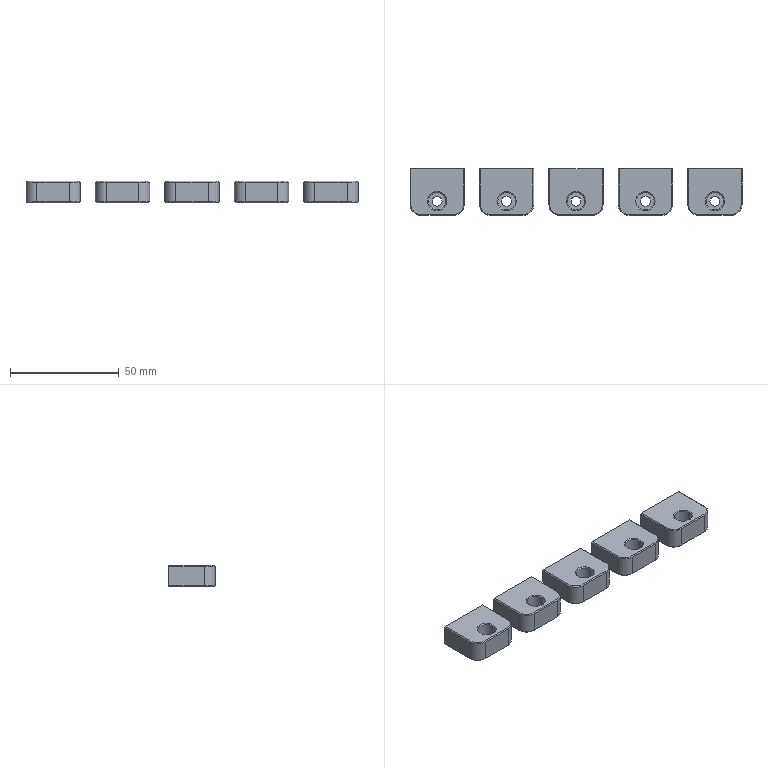NC program | NX | posted with a generic post | part box 153 x 21.5 x 10 mm
Whole program:
N10 G17 G21 G94 G90
(DRILLING_COPY_COPY , TOOL : D4A45)
N12 T02 M6
N14 G54
N16 G17 G0 G90 X-69. Y-5. B0. C0. S5000 M3
N18 G43 Z30. H2
N20 G94 G81 G98 Z-1.85 F250. R3.
N22 X-59.
N24 X-37.
N26 X-27.
N28 X-5.
N30 X5.
N32 X27.
N34 X37.
N36 X59.
N38 X69.
N40 G80
N42 G0 X69. Y-5. Z30.
N44 M5
(DRILLING_COPY_COPY_COPY_COPY_COPY_COPY_1 , TOOL : 3.5ZT)
N46 T15 M6
N48 G54
N50 G17 G0 G90 X-69. Y-5. B0. C0. S1910 M3
N52 G43 Z30. H15
N54 G94 G83 G98 Z-10.052 F180. Q2. R3.
N56 X-59.
N58 X-37.
N60 X-27.
N62 X-5.
N64 X5.
N66 X27.
N68 X37.
N70 X59.
N72 X69.
N74 G80
N76 G0 X69. Y-5. Z30.
N78 M5
N80 M2